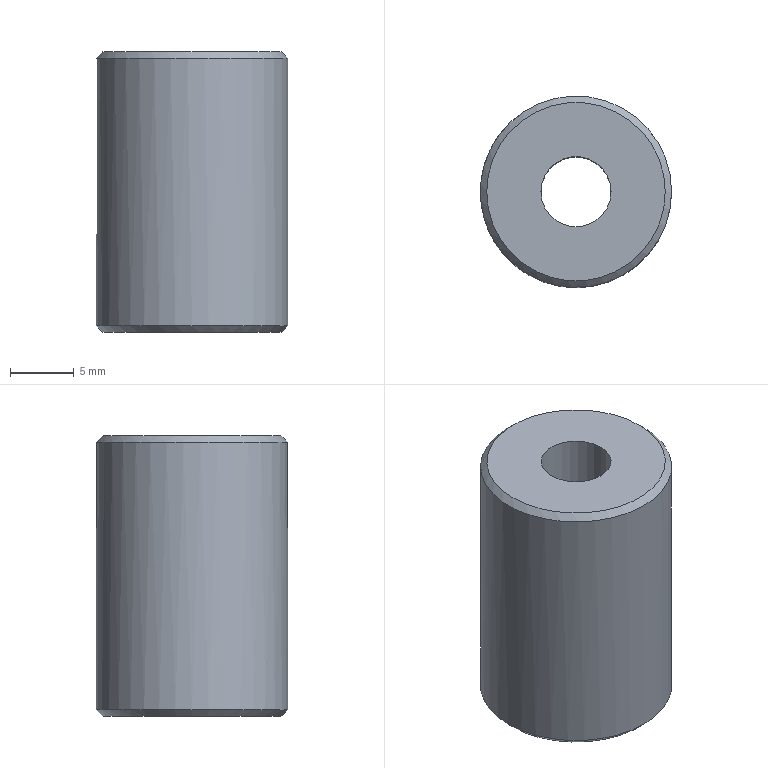Part | STEP file | Tube feed_id946_x_t | 1 solid | 6 faces | box 15 x 15 x 22 mm | volume 3354 mm3 | plane 2 | cylinder 2 | cone 2 | commonest cylinder face diameters 5.5 x1 15 x1
STEP:
#1=CARTESIAN_POINT('',(0.,0.,0.));
#2=DIRECTION('',(0.,0.,1.));
#3=DIRECTION('',(1.,0.,0.));
#4=AXIS2_PLACEMENT_3D('',#1,#2,#3);
#5=CARTESIAN_POINT('',(-192.,10.056,-86.4));
#6=VERTEX_POINT('',#5);
#7=CARTESIAN_POINT('',(-199.,10.056,-86.4));
#8=DIRECTION('',(0.,0.,1.));
#9=DIRECTION('',(1.,0.,0.));
#10=AXIS2_PLACEMENT_3D('',#7,#8,#9);
#11=CIRCLE('',#10,7.);
#12=CARTESIAN_POINT('',(-199.,10.056,-86.4));
#13=DIRECTION('',(0.,0.,1.));
#14=DIRECTION('',(1.,0.,0.));
#15=AXIS2_PLACEMENT_3D('',#12,#13,#14);
#16=PLANE('',#15);
#17=CARTESIAN_POINT('',(0.,0.));
#18=DIRECTION('',(1.,0.));
#19=AXIS2_PLACEMENT_2D('',#17,#18);
#20=CIRCLE('',#19,7.);
#21=(GEOMETRIC_REPRESENTATION_CONTEXT(2)PARAMETRIC_REPRESENTATION_CONTEXT()REPRESENTATION_CONTEXT('',''));
#22=DEFINITIONAL_REPRESENTATION('',(#20),#21);
#23=PCURVE('',#16,#22);
#24=CARTESIAN_POINT('',(-199.,10.056,-86.9));
#25=DIRECTION('',(0.,0.,-1.));
#26=DIRECTION('',(-1.,0.,0.));
#27=AXIS2_PLACEMENT_3D('',#24,#25,#26);
#28=CONICAL_SURFACE('',#27,7.5,0.7854);
#29=CARTESIAN_POINT('',(9.425,-0.5));
#30=DIRECTION('',(-1.,0.));
#31=VECTOR('',#30,1.);
#32=LINE('',#29,#31);
#33=(GEOMETRIC_REPRESENTATION_CONTEXT(2)PARAMETRIC_REPRESENTATION_CONTEXT()REPRESENTATION_CONTEXT('',''));
#34=DEFINITIONAL_REPRESENTATION('',(#32),#33);
#35=PCURVE('',#28,#34);
#36=SURFACE_CURVE('',#11,(#23,#35),.PCURVE_S1.);
#37=EDGE_CURVE('',#6,#6,#36,.T.);
#38=ORIENTED_EDGE('',*,*,#37,.T.);
#39=EDGE_LOOP('',(#38));
#40=FACE_BOUND('',#39,.T.);
#41=CARTESIAN_POINT('',(-201.75,10.056,-86.4));
#42=VERTEX_POINT('',#41);
#43=CARTESIAN_POINT('',(-199.,10.056,-86.4));
#44=DIRECTION('',(0.,0.,-1.));
#45=DIRECTION('',(-1.,0.,0.));
#46=AXIS2_PLACEMENT_3D('',#43,#44,#45);
#47=CIRCLE('',#46,2.75);
#48=CARTESIAN_POINT('',(-2.75,0.));
#49=CARTESIAN_POINT('',(-2.75,4.763));
#50=CARTESIAN_POINT('',(1.375,2.382));
#51=CARTESIAN_POINT('',(5.5,0.));
#52=CARTESIAN_POINT('',(1.375,-2.382));
#53=CARTESIAN_POINT('',(-2.75,-4.763));
#54=CARTESIAN_POINT('',(-2.75,0.));
#55=(BOUNDED_CURVE()B_SPLINE_CURVE(2,(#48,#49,#50,#51,#52,#53,#54),.UNSPECIFIED.,.T.,.F.)B_SPLINE_CURVE_WITH_KNOTS((1,2,2,2,2,1),(-2.094,0.,2.094,4.189,6.283,8.378),.UNSPECIFIED.)CURVE()GEOMETRIC_REPRESENTATION_ITEM()RATIONAL_B_SPLINE_CURVE((1.,0.5,1.,0.5,1.,0.5,1.))REPRESENTATION_ITEM(''));
#56=(GEOMETRIC_REPRESENTATION_CONTEXT(2)PARAMETRIC_REPRESENTATION_CONTEXT()REPRESENTATION_CONTEXT('',''));
#57=DEFINITIONAL_REPRESENTATION('',(#55),#56);
#58=PCURVE('',#16,#57);
#59=CARTESIAN_POINT('',(-199.,10.056,-86.4));
#60=DIRECTION('',(0.,0.,-1.));
#61=DIRECTION('',(-1.,0.,0.));
#62=AXIS2_PLACEMENT_3D('',#59,#60,#61);
#63=CYLINDRICAL_SURFACE('',#62,2.75);
#64=CARTESIAN_POINT('',(0.,0.));
#65=DIRECTION('',(1.,0.));
#66=VECTOR('',#65,1.);
#67=LINE('',#64,#66);
#68=(GEOMETRIC_REPRESENTATION_CONTEXT(2)PARAMETRIC_REPRESENTATION_CONTEXT()REPRESENTATION_CONTEXT('',''));
#69=DEFINITIONAL_REPRESENTATION('',(#67),#68);
#70=PCURVE('',#63,#69);
#71=SURFACE_CURVE('',#47,(#58,#70),.PCURVE_S1.);
#72=EDGE_CURVE('',#42,#42,#71,.T.);
#73=ORIENTED_EDGE('',*,*,#72,.T.);
#74=EDGE_LOOP('',(#73));
#75=FACE_BOUND('',#74,.T.);
#76=ADVANCED_FACE('',(#40,#75),#16,.T.);
#77=CARTESIAN_POINT('',(-206.,10.056,-108.4));
#78=VERTEX_POINT('',#77);
#79=CARTESIAN_POINT('',(-199.,10.056,-108.4));
#80=DIRECTION('',(0.,0.,-1.));
#81=DIRECTION('',(-1.,0.,0.));
#82=AXIS2_PLACEMENT_3D('',#79,#80,#81);
#83=CIRCLE('',#82,7.);
#84=CARTESIAN_POINT('',(-199.,10.056,-108.4));
#85=DIRECTION('',(0.,0.,-1.));
#86=DIRECTION('',(-1.,0.,0.));
#87=AXIS2_PLACEMENT_3D('',#84,#85,#86);
#88=PLANE('',#87);
#89=CARTESIAN_POINT('',(0.,0.));
#90=DIRECTION('',(1.,0.));
#91=AXIS2_PLACEMENT_2D('',#89,#90);
#92=CIRCLE('',#91,7.);
#93=(GEOMETRIC_REPRESENTATION_CONTEXT(2)PARAMETRIC_REPRESENTATION_CONTEXT()REPRESENTATION_CONTEXT('',''));
#94=DEFINITIONAL_REPRESENTATION('',(#92),#93);
#95=PCURVE('',#88,#94);
#96=CARTESIAN_POINT('',(-199.,10.056,-107.9));
#97=DIRECTION('',(0.,0.,1.));
#98=DIRECTION('',(1.,0.,0.));
#99=AXIS2_PLACEMENT_3D('',#96,#97,#98);
#100=CONICAL_SURFACE('',#99,7.5,0.7854);
#101=CARTESIAN_POINT('',(9.425,-0.5));
#102=DIRECTION('',(-1.,0.));
#103=VECTOR('',#102,1.);
#104=LINE('',#101,#103);
#105=(GEOMETRIC_REPRESENTATION_CONTEXT(2)PARAMETRIC_REPRESENTATION_CONTEXT()REPRESENTATION_CONTEXT('',''));
#106=DEFINITIONAL_REPRESENTATION('',(#104),#105);
#107=PCURVE('',#100,#106);
#108=SURFACE_CURVE('',#83,(#95,#107),.PCURVE_S1.);
#109=EDGE_CURVE('',#78,#78,#108,.T.);
#110=ORIENTED_EDGE('',*,*,#109,.T.);
#111=EDGE_LOOP('',(#110));
#112=FACE_BOUND('',#111,.T.);
#113=CARTESIAN_POINT('',(-201.75,10.056,-108.4));
#114=VERTEX_POINT('',#113);
#115=CARTESIAN_POINT('',(-199.,10.056,-108.4));
#116=DIRECTION('',(0.,0.,-1.));
#117=DIRECTION('',(-1.,0.,0.));
#118=AXIS2_PLACEMENT_3D('',#115,#116,#117);
#119=CIRCLE('',#118,2.75);
#120=CARTESIAN_POINT('',(0.,0.));
#121=DIRECTION('',(1.,0.));
#122=AXIS2_PLACEMENT_2D('',#120,#121);
#123=CIRCLE('',#122,2.75);
#124=(GEOMETRIC_REPRESENTATION_CONTEXT(2)PARAMETRIC_REPRESENTATION_CONTEXT()REPRESENTATION_CONTEXT('',''));
#125=DEFINITIONAL_REPRESENTATION('',(#123),#124);
#126=PCURVE('',#88,#125);
#127=CARTESIAN_POINT('',(0.,22.));
#128=DIRECTION('',(1.,0.));
#129=VECTOR('',#128,1.);
#130=LINE('',#127,#129);
#131=(GEOMETRIC_REPRESENTATION_CONTEXT(2)PARAMETRIC_REPRESENTATION_CONTEXT()REPRESENTATION_CONTEXT('',''));
#132=DEFINITIONAL_REPRESENTATION('',(#130),#131);
#133=PCURVE('',#63,#132);
#134=SURFACE_CURVE('',#119,(#126,#133),.PCURVE_S1.);
#135=EDGE_CURVE('',#114,#114,#134,.T.);
#136=ORIENTED_EDGE('',*,*,#135,.F.);
#137=EDGE_LOOP('',(#136));
#138=FACE_BOUND('',#137,.T.);
#139=ADVANCED_FACE('',(#112,#138),#88,.T.);
#140=CARTESIAN_POINT('',(-206.5,10.056,-107.9));
#141=VERTEX_POINT('',#140);
#142=CARTESIAN_POINT('',(-191.5,10.056,-107.9));
#143=VERTEX_POINT('',#142);
#144=CARTESIAN_POINT('',(-199.,10.056,-107.9));
#145=DIRECTION('',(0.,0.,1.));
#146=DIRECTION('',(-1.,0.,0.));
#147=AXIS2_PLACEMENT_3D('',#144,#145,#146);
#148=CIRCLE('',#147,7.5);
#149=CARTESIAN_POINT('',(-199.,10.056,-108.4));
#150=DIRECTION('',(0.,0.,1.));
#151=DIRECTION('',(1.,0.,0.));
#152=AXIS2_PLACEMENT_3D('',#149,#150,#151);
#153=CYLINDRICAL_SURFACE('',#152,7.5);
#154=CARTESIAN_POINT('',(3.142,0.5));
#155=DIRECTION('',(1.,0.));
#156=VECTOR('',#155,1.);
#157=LINE('',#154,#156);
#158=(GEOMETRIC_REPRESENTATION_CONTEXT(2)PARAMETRIC_REPRESENTATION_CONTEXT()REPRESENTATION_CONTEXT('',''));
#159=DEFINITIONAL_REPRESENTATION('',(#157),#158);
#160=PCURVE('',#153,#159);
#161=CARTESIAN_POINT('',(3.142,0.));
#162=DIRECTION('',(1.,0.));
#163=VECTOR('',#162,1.);
#164=LINE('',#161,#163);
#165=(GEOMETRIC_REPRESENTATION_CONTEXT(2)PARAMETRIC_REPRESENTATION_CONTEXT()REPRESENTATION_CONTEXT('',''));
#166=DEFINITIONAL_REPRESENTATION('',(#164),#165);
#167=PCURVE('',#100,#166);
#168=SURFACE_CURVE('',#148,(#160,#167),.PCURVE_S1.);
#169=EDGE_CURVE('',#141,#143,#168,.T.);
#170=ORIENTED_EDGE('',*,*,#169,.T.);
#171=CARTESIAN_POINT('',(-191.5,10.056,-86.9));
#172=VERTEX_POINT('',#171);
#173=CARTESIAN_POINT('',(-191.5,10.056,-107.9));
#174=CARTESIAN_POINT('',(-191.5,10.056,-86.9));
#175=B_SPLINE_CURVE_WITH_KNOTS('',1,(#173,#174),.UNSPECIFIED.,.F.,.F.,(2,2),(0.5,21.5),.PIECEWISE_BEZIER_KNOTS.);
#176=CARTESIAN_POINT('',(6.283,0.));
#177=DIRECTION('',(0.,1.));
#178=VECTOR('',#177,1.);
#179=LINE('',#176,#178);
#180=(GEOMETRIC_REPRESENTATION_CONTEXT(2)PARAMETRIC_REPRESENTATION_CONTEXT()REPRESENTATION_CONTEXT('',''));
#181=DEFINITIONAL_REPRESENTATION('',(#179),#180);
#182=PCURVE('',#153,#181);
#183=CARTESIAN_POINT('',(0.,0.));
#184=DIRECTION('',(0.,1.));
#185=VECTOR('',#184,1.);
#186=LINE('',#183,#185);
#187=(GEOMETRIC_REPRESENTATION_CONTEXT(2)PARAMETRIC_REPRESENTATION_CONTEXT()REPRESENTATION_CONTEXT('',''));
#188=DEFINITIONAL_REPRESENTATION('',(#186),#187);
#189=PCURVE('',#153,#188);
#190=SEAM_CURVE('',#175,(#182,#189),.PCURVE_S1.);
#191=EDGE_CURVE('',#143,#172,#190,.T.);
#192=ORIENTED_EDGE('',*,*,#191,.T.);
#193=CARTESIAN_POINT('',(-199.,10.056,-86.9));
#194=DIRECTION('',(0.,0.,-1.));
#195=DIRECTION('',(1.,0.,0.));
#196=AXIS2_PLACEMENT_3D('',#193,#194,#195);
#197=CIRCLE('',#196,7.5);
#198=CARTESIAN_POINT('',(6.283,21.5));
#199=DIRECTION('',(-1.,0.));
#200=VECTOR('',#199,1.);
#201=LINE('',#198,#200);
#202=(GEOMETRIC_REPRESENTATION_CONTEXT(2)PARAMETRIC_REPRESENTATION_CONTEXT()REPRESENTATION_CONTEXT('',''));
#203=DEFINITIONAL_REPRESENTATION('',(#201),#202);
#204=PCURVE('',#153,#203);
#205=CARTESIAN_POINT('',(3.142,0.));
#206=DIRECTION('',(1.,0.));
#207=VECTOR('',#206,1.);
#208=LINE('',#205,#207);
#209=(GEOMETRIC_REPRESENTATION_CONTEXT(2)PARAMETRIC_REPRESENTATION_CONTEXT()REPRESENTATION_CONTEXT('',''));
#210=DEFINITIONAL_REPRESENTATION('',(#208),#209);
#211=PCURVE('',#28,#210);
#212=SURFACE_CURVE('',#197,(#204,#211),.PCURVE_S1.);
#213=EDGE_CURVE('',#172,#172,#212,.T.);
#214=ORIENTED_EDGE('',*,*,#213,.T.);
#215=ORIENTED_EDGE('',*,*,#191,.F.);
#216=CARTESIAN_POINT('',(-199.,10.056,-107.9));
#217=DIRECTION('',(0.,0.,1.));
#218=DIRECTION('',(-1.,0.,0.));
#219=AXIS2_PLACEMENT_3D('',#216,#217,#218);
#220=CIRCLE('',#219,7.5);
#221=CARTESIAN_POINT('',(-3.142,0.5));
#222=DIRECTION('',(1.,0.));
#223=VECTOR('',#222,1.);
#224=LINE('',#221,#223);
#225=(GEOMETRIC_REPRESENTATION_CONTEXT(2)PARAMETRIC_REPRESENTATION_CONTEXT()REPRESENTATION_CONTEXT('',''));
#226=DEFINITIONAL_REPRESENTATION('',(#224),#225);
#227=PCURVE('',#153,#226);
#228=CARTESIAN_POINT('',(3.142,0.));
#229=DIRECTION('',(1.,0.));
#230=VECTOR('',#229,1.);
#231=LINE('',#228,#230);
#232=(GEOMETRIC_REPRESENTATION_CONTEXT(2)PARAMETRIC_REPRESENTATION_CONTEXT()REPRESENTATION_CONTEXT('',''));
#233=DEFINITIONAL_REPRESENTATION('',(#231),#232);
#234=PCURVE('',#100,#233);
#235=SURFACE_CURVE('',#220,(#227,#234),.PCURVE_S1.);
#236=EDGE_CURVE('',#143,#141,#235,.T.);
#237=ORIENTED_EDGE('',*,*,#236,.T.);
#238=EDGE_LOOP('',(#170,#192,#214,#215,#237));
#239=FACE_BOUND('',#238,.T.);
#240=ADVANCED_FACE('',(#239),#153,.T.);
#241=ORIENTED_EDGE('',*,*,#135,.F.);
#242=CARTESIAN_POINT('',(-201.75,10.056,-86.4));
#243=CARTESIAN_POINT('',(-201.75,10.056,-108.4));
#244=B_SPLINE_CURVE_WITH_KNOTS('',1,(#242,#243),.UNSPECIFIED.,.F.,.F.,(2,2),(0.,22.),.PIECEWISE_BEZIER_KNOTS.);
#245=CARTESIAN_POINT('',(0.,0.));
#246=DIRECTION('',(0.,1.));
#247=VECTOR('',#246,1.);
#248=LINE('',#245,#247);
#249=(GEOMETRIC_REPRESENTATION_CONTEXT(2)PARAMETRIC_REPRESENTATION_CONTEXT()REPRESENTATION_CONTEXT('',''));
#250=DEFINITIONAL_REPRESENTATION('',(#248),#249);
#251=PCURVE('',#63,#250);
#252=CARTESIAN_POINT('',(6.283,0.));
#253=DIRECTION('',(0.,1.));
#254=VECTOR('',#253,1.);
#255=LINE('',#252,#254);
#256=(GEOMETRIC_REPRESENTATION_CONTEXT(2)PARAMETRIC_REPRESENTATION_CONTEXT()REPRESENTATION_CONTEXT('',''));
#257=DEFINITIONAL_REPRESENTATION('',(#255),#256);
#258=PCURVE('',#63,#257);
#259=SEAM_CURVE('',#244,(#251,#258),.PCURVE_S1.);
#260=EDGE_CURVE('',#42,#114,#259,.T.);
#261=ORIENTED_EDGE('',*,*,#260,.F.);
#262=ORIENTED_EDGE('',*,*,#72,.T.);
#263=ORIENTED_EDGE('',*,*,#260,.T.);
#264=EDGE_LOOP('',(#241,#261,#262,#263));
#265=FACE_BOUND('',#264,.F.);
#266=ADVANCED_FACE('',(#265),#63,.F.);
#267=ORIENTED_EDGE('',*,*,#109,.F.);
#268=CARTESIAN_POINT('',(-206.,10.056,-108.4));
#269=CARTESIAN_POINT('',(-206.5,10.056,-107.9));
#270=B_SPLINE_CURVE_WITH_KNOTS('',1,(#268,#269),.UNSPECIFIED.,.F.,.F.,(2,2),(-0.7071,0.),.PIECEWISE_BEZIER_KNOTS.);
#271=CARTESIAN_POINT('',(9.425,0.));
#272=DIRECTION('',(0.,1.));
#273=VECTOR('',#272,1.);
#274=LINE('',#271,#273);
#275=(GEOMETRIC_REPRESENTATION_CONTEXT(2)PARAMETRIC_REPRESENTATION_CONTEXT()REPRESENTATION_CONTEXT('',''));
#276=DEFINITIONAL_REPRESENTATION('',(#274),#275);
#277=PCURVE('',#100,#276);
#278=CARTESIAN_POINT('',(3.142,0.));
#279=DIRECTION('',(0.,1.));
#280=VECTOR('',#279,1.);
#281=LINE('',#278,#280);
#282=(GEOMETRIC_REPRESENTATION_CONTEXT(2)PARAMETRIC_REPRESENTATION_CONTEXT()REPRESENTATION_CONTEXT('',''));
#283=DEFINITIONAL_REPRESENTATION('',(#281),#282);
#284=PCURVE('',#100,#283);
#285=SEAM_CURVE('',#270,(#277,#284),.PCURVE_S1.);
#286=EDGE_CURVE('',#78,#141,#285,.T.);
#287=ORIENTED_EDGE('',*,*,#286,.T.);
#288=ORIENTED_EDGE('',*,*,#236,.F.);
#289=ORIENTED_EDGE('',*,*,#169,.F.);
#290=ORIENTED_EDGE('',*,*,#286,.F.);
#291=EDGE_LOOP('',(#267,#287,#288,#289,#290));
#292=FACE_BOUND('',#291,.T.);
#293=ADVANCED_FACE('',(#292),#100,.T.);
#294=ORIENTED_EDGE('',*,*,#37,.F.);
#295=CARTESIAN_POINT('',(-192.,10.056,-86.4));
#296=CARTESIAN_POINT('',(-191.5,10.056,-86.9));
#297=B_SPLINE_CURVE_WITH_KNOTS('',1,(#295,#296),.UNSPECIFIED.,.F.,.F.,(2,2),(-0.7071,0.),.PIECEWISE_BEZIER_KNOTS.);
#298=CARTESIAN_POINT('',(9.425,0.));
#299=DIRECTION('',(0.,1.));
#300=VECTOR('',#299,1.);
#301=LINE('',#298,#300);
#302=(GEOMETRIC_REPRESENTATION_CONTEXT(2)PARAMETRIC_REPRESENTATION_CONTEXT()REPRESENTATION_CONTEXT('',''));
#303=DEFINITIONAL_REPRESENTATION('',(#301),#302);
#304=PCURVE('',#28,#303);
#305=CARTESIAN_POINT('',(3.142,0.));
#306=DIRECTION('',(0.,1.));
#307=VECTOR('',#306,1.);
#308=LINE('',#305,#307);
#309=(GEOMETRIC_REPRESENTATION_CONTEXT(2)PARAMETRIC_REPRESENTATION_CONTEXT()REPRESENTATION_CONTEXT('',''));
#310=DEFINITIONAL_REPRESENTATION('',(#308),#309);
#311=PCURVE('',#28,#310);
#312=SEAM_CURVE('',#297,(#304,#311),.PCURVE_S1.);
#313=EDGE_CURVE('',#6,#172,#312,.T.);
#314=ORIENTED_EDGE('',*,*,#313,.T.);
#315=ORIENTED_EDGE('',*,*,#213,.F.);
#316=ORIENTED_EDGE('',*,*,#313,.F.);
#317=EDGE_LOOP('',(#294,#314,#315,#316));
#318=FACE_BOUND('',#317,.T.);
#319=ADVANCED_FACE('',(#318),#28,.T.);
#320=CLOSED_SHELL('',(#76,#139,#240,#266,#293,#319));
#321=MANIFOLD_SOLID_BREP('',#320);
#322=(LENGTH_UNIT()NAMED_UNIT(*)SI_UNIT(.MILLI.,.METRE.));
#323=UNCERTAINTY_MEASURE_WITH_UNIT(LENGTH_MEASURE(0.00001),#322,'','');
#324=(NAMED_UNIT(*)PLANE_ANGLE_UNIT()SI_UNIT($,.RADIAN.));
#325=(NAMED_UNIT(*)SI_UNIT($,.STERADIAN.)SOLID_ANGLE_UNIT());
#326=(GEOMETRIC_REPRESENTATION_CONTEXT(3)GLOBAL_UNCERTAINTY_ASSIGNED_CONTEXT((#323))GLOBAL_UNIT_ASSIGNED_CONTEXT((#322,#324,#325))REPRESENTATION_CONTEXT('',''));
#327=ADVANCED_BREP_SHAPE_REPRESENTATION('',(#4,#321),#326);